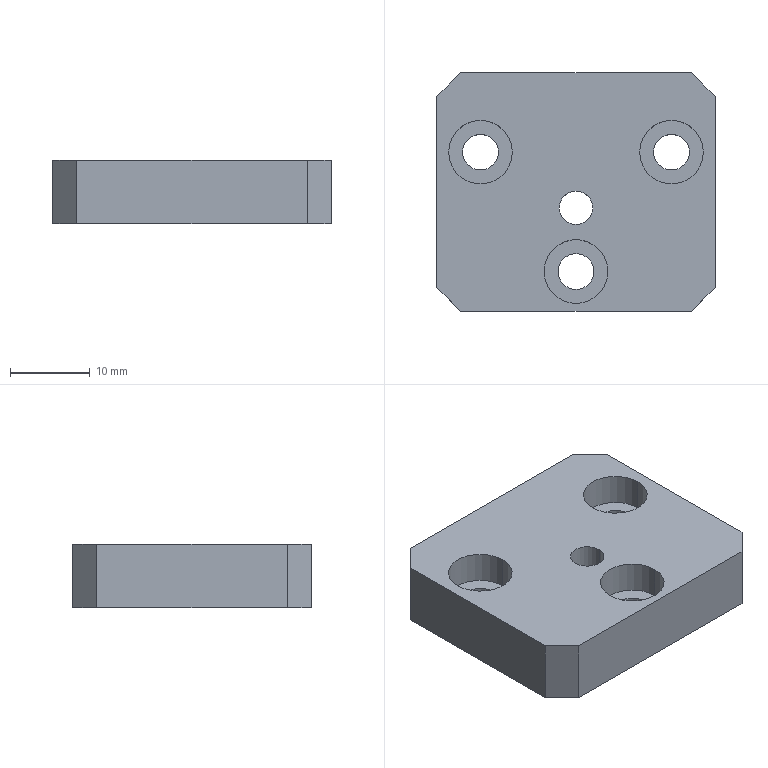Part | STEP file | pin seat 1 | 1 solid | 27 faces | box 35 x 30 x 8 mm | volume 7351 mm3 | cylinder 14 | plane 13 | commonest cylinder face diameters 4.5 x6 8 x6 4.2 x2